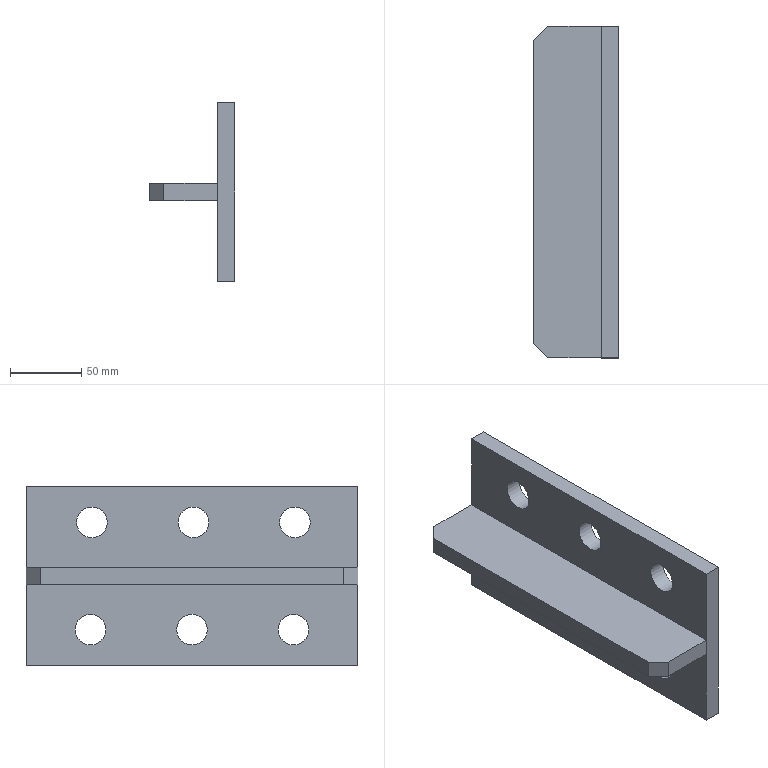Part | STEP file | PN_0039 web-top 12t steel corbel_Default<As Machined> | 2 solids | 20 faces | box 59.5 x 232 x 125 mm | volume 452900 mm3 | plane 14 | cylinder 6 | commonest cylinder face diameters 21.5 x6
STEP:
#1=CARTESIAN_POINT('',(0.,0.,0.));
#2=DIRECTION('',(0.,0.,1.));
#3=DIRECTION('',(1.,0.,0.));
#4=AXIS2_PLACEMENT_3D('',#1,#2,#3);
#5=CARTESIAN_POINT('',(23.75,-115.,-56.496));
#6=VERTEX_POINT('',#5);
#7=CARTESIAN_POINT('',(23.75,117.,-56.496));
#8=VERTEX_POINT('',#7);
#9=CARTESIAN_POINT('',(23.75,117.,-56.496));
#10=DIRECTION('',(0.,1.,0.));
#11=VECTOR('',#10,1.);
#12=LINE('',#9,#11);
#13=CARTESIAN_POINT('',(35.75,117.,-56.496));
#14=DIRECTION('',(0.,0.,1.));
#15=DIRECTION('',(0.,-1.,0.));
#16=AXIS2_PLACEMENT_3D('',#13,#14,#15);
#17=PLANE('',#16);
#18=CARTESIAN_POINT('',(0.,-12.));
#19=DIRECTION('',(-1.,0.));
#20=VECTOR('',#19,1.);
#21=LINE('',#18,#20);
#22=(GEOMETRIC_REPRESENTATION_CONTEXT(2)PARAMETRIC_REPRESENTATION_CONTEXT()REPRESENTATION_CONTEXT('',''));
#23=DEFINITIONAL_REPRESENTATION('',(#21),#22);
#24=PCURVE('',#17,#23);
#25=CARTESIAN_POINT('',(23.75,-17.06,106.06));
#26=DIRECTION('',(1.,0.,0.));
#27=DIRECTION('',(0.,0.,-1.));
#28=AXIS2_PLACEMENT_3D('',#25,#26,#27);
#29=PLANE('',#28);
#30=CARTESIAN_POINT('',(162.556,134.06));
#31=DIRECTION('',(0.,1.));
#32=VECTOR('',#31,1.);
#33=LINE('',#30,#32);
#34=(GEOMETRIC_REPRESENTATION_CONTEXT(2)PARAMETRIC_REPRESENTATION_CONTEXT()REPRESENTATION_CONTEXT('',''));
#35=DEFINITIONAL_REPRESENTATION('',(#33),#34);
#36=PCURVE('',#29,#35);
#37=SURFACE_CURVE('',#12,(#24,#36),.PCURVE_S1.);
#38=EDGE_CURVE('',#6,#8,#37,.T.);
#39=ORIENTED_EDGE('',*,*,#38,.T.);
#40=CARTESIAN_POINT('',(35.75,117.,-56.496));
#41=VERTEX_POINT('',#40);
#42=CARTESIAN_POINT('',(35.75,117.,-56.496));
#43=DIRECTION('',(-1.,0.,0.));
#44=VECTOR('',#43,1.);
#45=LINE('',#42,#44);
#46=CARTESIAN_POINT('',(0.,0.));
#47=DIRECTION('',(0.,-1.));
#48=VECTOR('',#47,1.);
#49=LINE('',#46,#48);
#50=(GEOMETRIC_REPRESENTATION_CONTEXT(2)PARAMETRIC_REPRESENTATION_CONTEXT()REPRESENTATION_CONTEXT('',''));
#51=DEFINITIONAL_REPRESENTATION('',(#49),#50);
#52=PCURVE('',#17,#51);
#53=CARTESIAN_POINT('',(35.75,117.,68.504));
#54=DIRECTION('',(0.,-1.,0.));
#55=DIRECTION('',(0.,0.,-1.));
#56=AXIS2_PLACEMENT_3D('',#53,#54,#55);
#57=PLANE('',#56);
#58=CARTESIAN_POINT('',(125.,0.));
#59=DIRECTION('',(0.,-1.));
#60=VECTOR('',#59,1.);
#61=LINE('',#58,#60);
#62=(GEOMETRIC_REPRESENTATION_CONTEXT(2)PARAMETRIC_REPRESENTATION_CONTEXT()REPRESENTATION_CONTEXT('',''));
#63=DEFINITIONAL_REPRESENTATION('',(#61),#62);
#64=PCURVE('',#57,#63);
#65=SURFACE_CURVE('',#45,(#52,#64),.PCURVE_S1.);
#66=EDGE_CURVE('',#41,#8,#65,.T.);
#67=ORIENTED_EDGE('',*,*,#66,.F.);
#68=CARTESIAN_POINT('',(35.75,-115.,-56.496));
#69=VERTEX_POINT('',#68);
#70=CARTESIAN_POINT('',(35.75,117.,-56.496));
#71=DIRECTION('',(0.,1.,0.));
#72=VECTOR('',#71,1.);
#73=LINE('',#70,#72);
#74=CARTESIAN_POINT('',(0.,0.));
#75=DIRECTION('',(-1.,0.));
#76=VECTOR('',#75,1.);
#77=LINE('',#74,#76);
#78=(GEOMETRIC_REPRESENTATION_CONTEXT(2)PARAMETRIC_REPRESENTATION_CONTEXT()REPRESENTATION_CONTEXT('',''));
#79=DEFINITIONAL_REPRESENTATION('',(#77),#78);
#80=PCURVE('',#17,#79);
#81=CARTESIAN_POINT('',(35.75,-17.06,106.06));
#82=DIRECTION('',(1.,0.,0.));
#83=DIRECTION('',(0.,0.,-1.));
#84=AXIS2_PLACEMENT_3D('',#81,#82,#83);
#85=PLANE('',#84);
#86=CARTESIAN_POINT('',(162.556,134.06));
#87=DIRECTION('',(0.,1.));
#88=VECTOR('',#87,1.);
#89=LINE('',#86,#88);
#90=(GEOMETRIC_REPRESENTATION_CONTEXT(2)PARAMETRIC_REPRESENTATION_CONTEXT()REPRESENTATION_CONTEXT('',''));
#91=DEFINITIONAL_REPRESENTATION('',(#89),#90);
#92=PCURVE('',#85,#91);
#93=SURFACE_CURVE('',#73,(#80,#92),.PCURVE_S1.);
#94=EDGE_CURVE('',#69,#41,#93,.T.);
#95=ORIENTED_EDGE('',*,*,#94,.F.);
#96=CARTESIAN_POINT('',(35.75,-115.,-56.496));
#97=DIRECTION('',(-1.,0.,0.));
#98=VECTOR('',#97,1.);
#99=LINE('',#96,#98);
#100=CARTESIAN_POINT('',(232.,0.));
#101=DIRECTION('',(0.,-1.));
#102=VECTOR('',#101,1.);
#103=LINE('',#100,#102);
#104=(GEOMETRIC_REPRESENTATION_CONTEXT(2)PARAMETRIC_REPRESENTATION_CONTEXT()REPRESENTATION_CONTEXT('',''));
#105=DEFINITIONAL_REPRESENTATION('',(#103),#104);
#106=PCURVE('',#17,#105);
#107=CARTESIAN_POINT('',(35.75,-115.,68.504));
#108=DIRECTION('',(0.,1.,0.));
#109=DIRECTION('',(0.,0.,1.));
#110=AXIS2_PLACEMENT_3D('',#107,#108,#109);
#111=PLANE('',#110);
#112=CARTESIAN_POINT('',(-125.,0.));
#113=DIRECTION('',(0.,-1.));
#114=VECTOR('',#113,1.);
#115=LINE('',#112,#114);
#116=(GEOMETRIC_REPRESENTATION_CONTEXT(2)PARAMETRIC_REPRESENTATION_CONTEXT()REPRESENTATION_CONTEXT('',''));
#117=DEFINITIONAL_REPRESENTATION('',(#115),#116);
#118=PCURVE('',#111,#117);
#119=SURFACE_CURVE('',#99,(#106,#118),.PCURVE_S1.);
#120=EDGE_CURVE('',#69,#6,#119,.T.);
#121=ORIENTED_EDGE('',*,*,#120,.T.);
#122=EDGE_LOOP('',(#39,#67,#95,#121));
#123=FACE_BOUND('',#122,.T.);
#124=ADVANCED_FACE('',(#123),#17,.F.);
#125=CARTESIAN_POINT('',(23.75,117.,68.504));
#126=VERTEX_POINT('',#125);
#127=CARTESIAN_POINT('',(23.75,117.,68.504));
#128=DIRECTION('',(0.,0.,1.));
#129=VECTOR('',#128,1.);
#130=LINE('',#127,#129);
#131=CARTESIAN_POINT('',(0.,-12.));
#132=DIRECTION('',(-1.,0.));
#133=VECTOR('',#132,1.);
#134=LINE('',#131,#133);
#135=(GEOMETRIC_REPRESENTATION_CONTEXT(2)PARAMETRIC_REPRESENTATION_CONTEXT()REPRESENTATION_CONTEXT('',''));
#136=DEFINITIONAL_REPRESENTATION('',(#134),#135);
#137=PCURVE('',#57,#136);
#138=CARTESIAN_POINT('',(37.556,134.06));
#139=DIRECTION('',(-1.,0.));
#140=VECTOR('',#139,1.);
#141=LINE('',#138,#140);
#142=(GEOMETRIC_REPRESENTATION_CONTEXT(2)PARAMETRIC_REPRESENTATION_CONTEXT()REPRESENTATION_CONTEXT('',''));
#143=DEFINITIONAL_REPRESENTATION('',(#141),#142);
#144=PCURVE('',#29,#143);
#145=SURFACE_CURVE('',#130,(#137,#144),.PCURVE_S1.);
#146=EDGE_CURVE('',#8,#126,#145,.T.);
#147=ORIENTED_EDGE('',*,*,#146,.T.);
#148=CARTESIAN_POINT('',(35.75,117.,68.504));
#149=VERTEX_POINT('',#148);
#150=CARTESIAN_POINT('',(35.75,117.,68.504));
#151=DIRECTION('',(-1.,0.,0.));
#152=VECTOR('',#151,1.);
#153=LINE('',#150,#152);
#154=CARTESIAN_POINT('',(0.,0.));
#155=DIRECTION('',(0.,-1.));
#156=VECTOR('',#155,1.);
#157=LINE('',#154,#156);
#158=(GEOMETRIC_REPRESENTATION_CONTEXT(2)PARAMETRIC_REPRESENTATION_CONTEXT()REPRESENTATION_CONTEXT('',''));
#159=DEFINITIONAL_REPRESENTATION('',(#157),#158);
#160=PCURVE('',#57,#159);
#161=CARTESIAN_POINT('',(35.75,117.,68.504));
#162=DIRECTION('',(0.,0.,-1.));
#163=DIRECTION('',(0.,1.,0.));
#164=AXIS2_PLACEMENT_3D('',#161,#162,#163);
#165=PLANE('',#164);
#166=CARTESIAN_POINT('',(0.,0.));
#167=DIRECTION('',(0.,-1.));
#168=VECTOR('',#167,1.);
#169=LINE('',#166,#168);
#170=(GEOMETRIC_REPRESENTATION_CONTEXT(2)PARAMETRIC_REPRESENTATION_CONTEXT()REPRESENTATION_CONTEXT('',''));
#171=DEFINITIONAL_REPRESENTATION('',(#169),#170);
#172=PCURVE('',#165,#171);
#173=SURFACE_CURVE('',#153,(#160,#172),.PCURVE_S1.);
#174=EDGE_CURVE('',#149,#126,#173,.T.);
#175=ORIENTED_EDGE('',*,*,#174,.F.);
#176=CARTESIAN_POINT('',(35.75,117.,68.504));
#177=DIRECTION('',(0.,0.,1.));
#178=VECTOR('',#177,1.);
#179=LINE('',#176,#178);
#180=CARTESIAN_POINT('',(0.,0.));
#181=DIRECTION('',(-1.,0.));
#182=VECTOR('',#181,1.);
#183=LINE('',#180,#182);
#184=(GEOMETRIC_REPRESENTATION_CONTEXT(2)PARAMETRIC_REPRESENTATION_CONTEXT()REPRESENTATION_CONTEXT('',''));
#185=DEFINITIONAL_REPRESENTATION('',(#183),#184);
#186=PCURVE('',#57,#185);
#187=CARTESIAN_POINT('',(37.556,134.06));
#188=DIRECTION('',(-1.,0.));
#189=VECTOR('',#188,1.);
#190=LINE('',#187,#189);
#191=(GEOMETRIC_REPRESENTATION_CONTEXT(2)PARAMETRIC_REPRESENTATION_CONTEXT()REPRESENTATION_CONTEXT('',''));
#192=DEFINITIONAL_REPRESENTATION('',(#190),#191);
#193=PCURVE('',#85,#192);
#194=SURFACE_CURVE('',#179,(#186,#193),.PCURVE_S1.);
#195=EDGE_CURVE('',#41,#149,#194,.T.);
#196=ORIENTED_EDGE('',*,*,#195,.F.);
#197=ORIENTED_EDGE('',*,*,#66,.T.);
#198=EDGE_LOOP('',(#147,#175,#196,#197));
#199=FACE_BOUND('',#198,.T.);
#200=ADVANCED_FACE('',(#199),#57,.F.);
#201=CARTESIAN_POINT('',(23.75,-115.,68.504));
#202=VERTEX_POINT('',#201);
#203=CARTESIAN_POINT('',(23.75,117.,68.504));
#204=DIRECTION('',(0.,-1.,0.));
#205=VECTOR('',#204,1.);
#206=LINE('',#203,#205);
#207=CARTESIAN_POINT('',(0.,-12.));
#208=DIRECTION('',(-1.,0.));
#209=VECTOR('',#208,1.);
#210=LINE('',#207,#209);
#211=(GEOMETRIC_REPRESENTATION_CONTEXT(2)PARAMETRIC_REPRESENTATION_CONTEXT()REPRESENTATION_CONTEXT('',''));
#212=DEFINITIONAL_REPRESENTATION('',(#210),#211);
#213=PCURVE('',#165,#212);
#214=CARTESIAN_POINT('',(37.556,134.06));
#215=DIRECTION('',(0.,-1.));
#216=VECTOR('',#215,1.);
#217=LINE('',#214,#216);
#218=(GEOMETRIC_REPRESENTATION_CONTEXT(2)PARAMETRIC_REPRESENTATION_CONTEXT()REPRESENTATION_CONTEXT('',''));
#219=DEFINITIONAL_REPRESENTATION('',(#217),#218);
#220=PCURVE('',#29,#219);
#221=SURFACE_CURVE('',#206,(#213,#220),.PCURVE_S1.);
#222=EDGE_CURVE('',#126,#202,#221,.T.);
#223=ORIENTED_EDGE('',*,*,#222,.T.);
#224=CARTESIAN_POINT('',(35.75,-115.,68.504));
#225=VERTEX_POINT('',#224);
#226=CARTESIAN_POINT('',(35.75,-115.,68.504));
#227=DIRECTION('',(-1.,0.,0.));
#228=VECTOR('',#227,1.);
#229=LINE('',#226,#228);
#230=CARTESIAN_POINT('',(-232.,0.));
#231=DIRECTION('',(0.,-1.));
#232=VECTOR('',#231,1.);
#233=LINE('',#230,#232);
#234=(GEOMETRIC_REPRESENTATION_CONTEXT(2)PARAMETRIC_REPRESENTATION_CONTEXT()REPRESENTATION_CONTEXT('',''));
#235=DEFINITIONAL_REPRESENTATION('',(#233),#234);
#236=PCURVE('',#165,#235);
#237=CARTESIAN_POINT('',(0.,0.));
#238=DIRECTION('',(0.,-1.));
#239=VECTOR('',#238,1.);
#240=LINE('',#237,#239);
#241=(GEOMETRIC_REPRESENTATION_CONTEXT(2)PARAMETRIC_REPRESENTATION_CONTEXT()REPRESENTATION_CONTEXT('',''));
#242=DEFINITIONAL_REPRESENTATION('',(#240),#241);
#243=PCURVE('',#111,#242);
#244=SURFACE_CURVE('',#229,(#236,#243),.PCURVE_S1.);
#245=EDGE_CURVE('',#225,#202,#244,.T.);
#246=ORIENTED_EDGE('',*,*,#245,.F.);
#247=CARTESIAN_POINT('',(35.75,117.,68.504));
#248=DIRECTION('',(0.,-1.,0.));
#249=VECTOR('',#248,1.);
#250=LINE('',#247,#249);
#251=CARTESIAN_POINT('',(0.,0.));
#252=DIRECTION('',(-1.,0.));
#253=VECTOR('',#252,1.);
#254=LINE('',#251,#253);
#255=(GEOMETRIC_REPRESENTATION_CONTEXT(2)PARAMETRIC_REPRESENTATION_CONTEXT()REPRESENTATION_CONTEXT('',''));
#256=DEFINITIONAL_REPRESENTATION('',(#254),#255);
#257=PCURVE('',#165,#256);
#258=CARTESIAN_POINT('',(37.556,134.06));
#259=DIRECTION('',(0.,-1.));
#260=VECTOR('',#259,1.);
#261=LINE('',#258,#260);
#262=(GEOMETRIC_REPRESENTATION_CONTEXT(2)PARAMETRIC_REPRESENTATION_CONTEXT()REPRESENTATION_CONTEXT('',''));
#263=DEFINITIONAL_REPRESENTATION('',(#261),#262);
#264=PCURVE('',#85,#263);
#265=SURFACE_CURVE('',#250,(#257,#264),.PCURVE_S1.);
#266=EDGE_CURVE('',#149,#225,#265,.T.);
#267=ORIENTED_EDGE('',*,*,#266,.F.);
#268=ORIENTED_EDGE('',*,*,#174,.T.);
#269=EDGE_LOOP('',(#223,#246,#267,#268));
#270=FACE_BOUND('',#269,.T.);
#271=ADVANCED_FACE('',(#270),#165,.F.);
#272=CARTESIAN_POINT('',(23.75,-115.,68.504));
#273=DIRECTION('',(0.,0.,-1.));
#274=VECTOR('',#273,1.);
#275=LINE('',#272,#274);
#276=CARTESIAN_POINT('',(0.,-12.));
#277=DIRECTION('',(-1.,0.));
#278=VECTOR('',#277,1.);
#279=LINE('',#276,#278);
#280=(GEOMETRIC_REPRESENTATION_CONTEXT(2)PARAMETRIC_REPRESENTATION_CONTEXT()REPRESENTATION_CONTEXT('',''));
#281=DEFINITIONAL_REPRESENTATION('',(#279),#280);
#282=PCURVE('',#111,#281);
#283=CARTESIAN_POINT('',(37.556,-97.94));
#284=DIRECTION('',(1.,0.));
#285=VECTOR('',#284,1.);
#286=LINE('',#283,#285);
#287=(GEOMETRIC_REPRESENTATION_CONTEXT(2)PARAMETRIC_REPRESENTATION_CONTEXT()REPRESENTATION_CONTEXT('',''));
#288=DEFINITIONAL_REPRESENTATION('',(#286),#287);
#289=PCURVE('',#29,#288);
#290=SURFACE_CURVE('',#275,(#282,#289),.PCURVE_S1.);
#291=EDGE_CURVE('',#202,#6,#290,.T.);
#292=ORIENTED_EDGE('',*,*,#291,.T.);
#293=ORIENTED_EDGE('',*,*,#120,.F.);
#294=CARTESIAN_POINT('',(35.75,-115.,68.504));
#295=DIRECTION('',(0.,0.,-1.));
#296=VECTOR('',#295,1.);
#297=LINE('',#294,#296);
#298=CARTESIAN_POINT('',(0.,0.));
#299=DIRECTION('',(-1.,0.));
#300=VECTOR('',#299,1.);
#301=LINE('',#298,#300);
#302=(GEOMETRIC_REPRESENTATION_CONTEXT(2)PARAMETRIC_REPRESENTATION_CONTEXT()REPRESENTATION_CONTEXT('',''));
#303=DEFINITIONAL_REPRESENTATION('',(#301),#302);
#304=PCURVE('',#111,#303);
#305=CARTESIAN_POINT('',(37.556,-97.94));
#306=DIRECTION('',(1.,0.));
#307=VECTOR('',#306,1.);
#308=LINE('',#305,#307);
#309=(GEOMETRIC_REPRESENTATION_CONTEXT(2)PARAMETRIC_REPRESENTATION_CONTEXT()REPRESENTATION_CONTEXT('',''));
#310=DEFINITIONAL_REPRESENTATION('',(#308),#309);
#311=PCURVE('',#85,#310);
#312=SURFACE_CURVE('',#297,(#304,#311),.PCURVE_S1.);
#313=EDGE_CURVE('',#225,#69,#312,.T.);
#314=ORIENTED_EDGE('',*,*,#313,.F.);
#315=ORIENTED_EDGE('',*,*,#245,.T.);
#316=EDGE_LOOP('',(#292,#293,#314,#315));
#317=FACE_BOUND('',#316,.T.);
#318=ADVANCED_FACE('',(#317),#111,.F.);
#319=CARTESIAN_POINT('',(35.75,71.,32.754));
#320=VERTEX_POINT('',#319);
#321=CARTESIAN_POINT('',(35.75,71.,43.504));
#322=DIRECTION('',(1.,0.,0.));
#323=DIRECTION('',(0.,0.,-1.));
#324=AXIS2_PLACEMENT_3D('',#321,#322,#323);
#325=CIRCLE('',#324,10.75);
#326=CARTESIAN_POINT('',(62.556,88.06));
#327=DIRECTION('',(1.,0.));
#328=AXIS2_PLACEMENT_2D('',#326,#327);
#329=CIRCLE('',#328,10.75);
#330=(GEOMETRIC_REPRESENTATION_CONTEXT(2)PARAMETRIC_REPRESENTATION_CONTEXT()REPRESENTATION_CONTEXT('',''));
#331=DEFINITIONAL_REPRESENTATION('',(#329),#330);
#332=PCURVE('',#85,#331);
#333=CARTESIAN_POINT('',(35.75,71.,43.504));
#334=DIRECTION('',(1.,0.,0.));
#335=DIRECTION('',(0.,0.,-1.));
#336=AXIS2_PLACEMENT_3D('',#333,#334,#335);
#337=CYLINDRICAL_SURFACE('',#336,10.75);
#338=CARTESIAN_POINT('',(0.,0.));
#339=DIRECTION('',(1.,0.));
#340=VECTOR('',#339,1.);
#341=LINE('',#338,#340);
#342=(GEOMETRIC_REPRESENTATION_CONTEXT(2)PARAMETRIC_REPRESENTATION_CONTEXT()REPRESENTATION_CONTEXT('',''));
#343=DEFINITIONAL_REPRESENTATION('',(#341),#342);
#344=PCURVE('',#337,#343);
#345=SURFACE_CURVE('',#325,(#332,#344),.PCURVE_S1.);
#346=EDGE_CURVE('',#320,#320,#345,.T.);
#347=ORIENTED_EDGE('',*,*,#346,.F.);
#348=EDGE_LOOP('',(#347));
#349=FACE_BOUND('',#348,.T.);
#350=CARTESIAN_POINT('',(35.75,0.0001482,32.754));
#351=VERTEX_POINT('',#350);
#352=CARTESIAN_POINT('',(35.75,0.0001482,43.504));
#353=DIRECTION('',(1.,0.,0.));
#354=DIRECTION('',(0.,0.,-1.));
#355=AXIS2_PLACEMENT_3D('',#352,#353,#354);
#356=CIRCLE('',#355,10.75);
#357=CARTESIAN_POINT('',(62.556,17.06));
#358=DIRECTION('',(1.,0.));
#359=AXIS2_PLACEMENT_2D('',#357,#358);
#360=CIRCLE('',#359,10.75);
#361=(GEOMETRIC_REPRESENTATION_CONTEXT(2)PARAMETRIC_REPRESENTATION_CONTEXT()REPRESENTATION_CONTEXT('',''));
#362=DEFINITIONAL_REPRESENTATION('',(#360),#361);
#363=PCURVE('',#85,#362);
#364=CARTESIAN_POINT('',(35.75,0.0001482,43.504));
#365=DIRECTION('',(1.,0.,0.));
#366=DIRECTION('',(0.,0.,-1.));
#367=AXIS2_PLACEMENT_3D('',#364,#365,#366);
#368=CYLINDRICAL_SURFACE('',#367,10.75);
#369=CARTESIAN_POINT('',(0.,0.));
#370=DIRECTION('',(1.,0.));
#371=VECTOR('',#370,1.);
#372=LINE('',#369,#371);
#373=(GEOMETRIC_REPRESENTATION_CONTEXT(2)PARAMETRIC_REPRESENTATION_CONTEXT()REPRESENTATION_CONTEXT('',''));
#374=DEFINITIONAL_REPRESENTATION('',(#372),#373);
#375=PCURVE('',#368,#374);
#376=SURFACE_CURVE('',#356,(#363,#375),.PCURVE_S1.);
#377=EDGE_CURVE('',#351,#351,#376,.T.);
#378=ORIENTED_EDGE('',*,*,#377,.F.);
#379=EDGE_LOOP('',(#378));
#380=FACE_BOUND('',#379,.T.);
#381=CARTESIAN_POINT('',(35.75,1.,-42.246));
#382=VERTEX_POINT('',#381);
#383=CARTESIAN_POINT('',(35.75,1.,-31.496));
#384=DIRECTION('',(1.,0.,0.));
#385=DIRECTION('',(0.,0.,-1.));
#386=AXIS2_PLACEMENT_3D('',#383,#384,#385);
#387=CIRCLE('',#386,10.75);
#388=CARTESIAN_POINT('',(137.556,18.06));
#389=DIRECTION('',(1.,0.));
#390=AXIS2_PLACEMENT_2D('',#388,#389);
#391=CIRCLE('',#390,10.75);
#392=(GEOMETRIC_REPRESENTATION_CONTEXT(2)PARAMETRIC_REPRESENTATION_CONTEXT()REPRESENTATION_CONTEXT('',''));
#393=DEFINITIONAL_REPRESENTATION('',(#391),#392);
#394=PCURVE('',#85,#393);
#395=CARTESIAN_POINT('',(35.75,1.,-31.496));
#396=DIRECTION('',(1.,0.,0.));
#397=DIRECTION('',(0.,0.,-1.));
#398=AXIS2_PLACEMENT_3D('',#395,#396,#397);
#399=CYLINDRICAL_SURFACE('',#398,10.75);
#400=CARTESIAN_POINT('',(0.,0.));
#401=DIRECTION('',(1.,0.));
#402=VECTOR('',#401,1.);
#403=LINE('',#400,#402);
#404=(GEOMETRIC_REPRESENTATION_CONTEXT(2)PARAMETRIC_REPRESENTATION_CONTEXT()REPRESENTATION_CONTEXT('',''));
#405=DEFINITIONAL_REPRESENTATION('',(#403),#404);
#406=PCURVE('',#399,#405);
#407=SURFACE_CURVE('',#387,(#394,#406),.PCURVE_S1.);
#408=EDGE_CURVE('',#382,#382,#407,.T.);
#409=ORIENTED_EDGE('',*,*,#408,.F.);
#410=EDGE_LOOP('',(#409));
#411=FACE_BOUND('',#410,.T.);
#412=CARTESIAN_POINT('',(35.75,72.,-42.246));
#413=VERTEX_POINT('',#412);
#414=CARTESIAN_POINT('',(35.75,72.,-31.496));
#415=DIRECTION('',(1.,0.,0.));
#416=DIRECTION('',(0.,0.,-1.));
#417=AXIS2_PLACEMENT_3D('',#414,#415,#416);
#418=CIRCLE('',#417,10.75);
#419=CARTESIAN_POINT('',(137.556,89.06));
#420=DIRECTION('',(1.,0.));
#421=AXIS2_PLACEMENT_2D('',#419,#420);
#422=CIRCLE('',#421,10.75);
#423=(GEOMETRIC_REPRESENTATION_CONTEXT(2)PARAMETRIC_REPRESENTATION_CONTEXT()REPRESENTATION_CONTEXT('',''));
#424=DEFINITIONAL_REPRESENTATION('',(#422),#423);
#425=PCURVE('',#85,#424);
#426=CARTESIAN_POINT('',(35.75,72.,-31.496));
#427=DIRECTION('',(1.,0.,0.));
#428=DIRECTION('',(0.,0.,-1.));
#429=AXIS2_PLACEMENT_3D('',#426,#427,#428);
#430=CYLINDRICAL_SURFACE('',#429,10.75);
#431=CARTESIAN_POINT('',(0.,0.));
#432=DIRECTION('',(1.,0.));
#433=VECTOR('',#432,1.);
#434=LINE('',#431,#433);
#435=(GEOMETRIC_REPRESENTATION_CONTEXT(2)PARAMETRIC_REPRESENTATION_CONTEXT()REPRESENTATION_CONTEXT('',''));
#436=DEFINITIONAL_REPRESENTATION('',(#434),#435);
#437=PCURVE('',#430,#436);
#438=SURFACE_CURVE('',#418,(#425,#437),.PCURVE_S1.);
#439=EDGE_CURVE('',#413,#413,#438,.T.);
#440=ORIENTED_EDGE('',*,*,#439,.F.);
#441=EDGE_LOOP('',(#440));
#442=FACE_BOUND('',#441,.T.);
#443=CARTESIAN_POINT('',(35.75,-71.,32.754));
#444=VERTEX_POINT('',#443);
#445=CARTESIAN_POINT('',(35.75,-71.,43.504));
#446=DIRECTION('',(1.,0.,0.));
#447=DIRECTION('',(0.,0.,-1.));
#448=AXIS2_PLACEMENT_3D('',#445,#446,#447);
#449=CIRCLE('',#448,10.75);
#450=CARTESIAN_POINT('',(62.556,-53.94));
#451=DIRECTION('',(1.,0.));
#452=AXIS2_PLACEMENT_2D('',#450,#451);
#453=CIRCLE('',#452,10.75);
#454=(GEOMETRIC_REPRESENTATION_CONTEXT(2)PARAMETRIC_REPRESENTATION_CONTEXT()REPRESENTATION_CONTEXT('',''));
#455=DEFINITIONAL_REPRESENTATION('',(#453),#454);
#456=PCURVE('',#85,#455);
#457=CARTESIAN_POINT('',(35.75,-71.,43.504));
#458=DIRECTION('',(1.,0.,0.));
#459=DIRECTION('',(0.,0.,-1.));
#460=AXIS2_PLACEMENT_3D('',#457,#458,#459);
#461=CYLINDRICAL_SURFACE('',#460,10.75);
#462=CARTESIAN_POINT('',(0.,0.));
#463=DIRECTION('',(1.,0.));
#464=VECTOR('',#463,1.);
#465=LINE('',#462,#464);
#466=(GEOMETRIC_REPRESENTATION_CONTEXT(2)PARAMETRIC_REPRESENTATION_CONTEXT()REPRESENTATION_CONTEXT('',''));
#467=DEFINITIONAL_REPRESENTATION('',(#465),#466);
#468=PCURVE('',#461,#467);
#469=SURFACE_CURVE('',#449,(#456,#468),.PCURVE_S1.);
#470=EDGE_CURVE('',#444,#444,#469,.T.);
#471=ORIENTED_EDGE('',*,*,#470,.F.);
#472=EDGE_LOOP('',(#471));
#473=FACE_BOUND('',#472,.T.);
#474=CARTESIAN_POINT('',(35.75,-70.,-42.246));
#475=VERTEX_POINT('',#474);
#476=CARTESIAN_POINT('',(35.75,-70.,-31.496));
#477=DIRECTION('',(1.,0.,0.));
#478=DIRECTION('',(0.,0.,-1.));
#479=AXIS2_PLACEMENT_3D('',#476,#477,#478);
#480=CIRCLE('',#479,10.75);
#481=CARTESIAN_POINT('',(137.556,-52.94));
#482=DIRECTION('',(1.,0.));
#483=AXIS2_PLACEMENT_2D('',#481,#482);
#484=CIRCLE('',#483,10.75);
#485=(GEOMETRIC_REPRESENTATION_CONTEXT(2)PARAMETRIC_REPRESENTATION_CONTEXT()REPRESENTATION_CONTEXT('',''));
#486=DEFINITIONAL_REPRESENTATION('',(#484),#485);
#487=PCURVE('',#85,#486);
#488=CARTESIAN_POINT('',(35.75,-70.,-31.496));
#489=DIRECTION('',(1.,0.,0.));
#490=DIRECTION('',(0.,0.,-1.));
#491=AXIS2_PLACEMENT_3D('',#488,#489,#490);
#492=CYLINDRICAL_SURFACE('',#491,10.75);
#493=CARTESIAN_POINT('',(0.,0.));
#494=DIRECTION('',(1.,0.));
#495=VECTOR('',#494,1.);
#496=LINE('',#493,#495);
#497=(GEOMETRIC_REPRESENTATION_CONTEXT(2)PARAMETRIC_REPRESENTATION_CONTEXT()REPRESENTATION_CONTEXT('',''));
#498=DEFINITIONAL_REPRESENTATION('',(#496),#497);
#499=PCURVE('',#492,#498);
#500=SURFACE_CURVE('',#480,(#487,#499),.PCURVE_S1.);
#501=EDGE_CURVE('',#475,#475,#500,.T.);
#502=ORIENTED_EDGE('',*,*,#501,.F.);
#503=EDGE_LOOP('',(#502));
#504=FACE_BOUND('',#503,.T.);
#505=ORIENTED_EDGE('',*,*,#94,.T.);
#506=ORIENTED_EDGE('',*,*,#195,.T.);
#507=ORIENTED_EDGE('',*,*,#266,.T.);
#508=ORIENTED_EDGE('',*,*,#313,.T.);
#509=EDGE_LOOP('',(#505,#506,#507,#508));
#510=FACE_BOUND('',#509,.T.);
#511=ADVANCED_FACE('',(#349,#380,#411,#442,#473,#504,#510),#85,.T.);
#512=CARTESIAN_POINT('',(23.75,71.,32.754));
#513=VERTEX_POINT('',#512);
#514=CARTESIAN_POINT('',(23.75,71.,43.504));
#515=DIRECTION('',(1.,0.,0.));
#516=DIRECTION('',(0.,0.,-1.));
#517=AXIS2_PLACEMENT_3D('',#514,#515,#516);
#518=CIRCLE('',#517,10.75);
#519=CARTESIAN_POINT('',(62.556,88.06));
#520=DIRECTION('',(1.,0.));
#521=AXIS2_PLACEMENT_2D('',#519,#520);
#522=CIRCLE('',#521,10.75);
#523=(GEOMETRIC_REPRESENTATION_CONTEXT(2)PARAMETRIC_REPRESENTATION_CONTEXT()REPRESENTATION_CONTEXT('',''));
#524=DEFINITIONAL_REPRESENTATION('',(#522),#523);
#525=PCURVE('',#29,#524);
#526=CARTESIAN_POINT('',(0.,-12.));
#527=DIRECTION('',(1.,0.));
#528=VECTOR('',#527,1.);
#529=LINE('',#526,#528);
#530=(GEOMETRIC_REPRESENTATION_CONTEXT(2)PARAMETRIC_REPRESENTATION_CONTEXT()REPRESENTATION_CONTEXT('',''));
#531=DEFINITIONAL_REPRESENTATION('',(#529),#530);
#532=PCURVE('',#337,#531);
#533=SURFACE_CURVE('',#518,(#525,#532),.PCURVE_S1.);
#534=EDGE_CURVE('',#513,#513,#533,.T.);
#535=ORIENTED_EDGE('',*,*,#534,.T.);
#536=EDGE_LOOP('',(#535));
#537=FACE_BOUND('',#536,.T.);
#538=CARTESIAN_POINT('',(23.75,0.0001482,32.754));
#539=VERTEX_POINT('',#538);
#540=CARTESIAN_POINT('',(23.75,0.0001482,43.504));
#541=DIRECTION('',(1.,0.,0.));
#542=DIRECTION('',(0.,0.,-1.));
#543=AXIS2_PLACEMENT_3D('',#540,#541,#542);
#544=CIRCLE('',#543,10.75);
#545=CARTESIAN_POINT('',(62.556,17.06));
#546=DIRECTION('',(1.,0.));
#547=AXIS2_PLACEMENT_2D('',#545,#546);
#548=CIRCLE('',#547,10.75);
#549=(GEOMETRIC_REPRESENTATION_CONTEXT(2)PARAMETRIC_REPRESENTATION_CONTEXT()REPRESENTATION_CONTEXT('',''));
#550=DEFINITIONAL_REPRESENTATION('',(#548),#549);
#551=PCURVE('',#29,#550);
#552=CARTESIAN_POINT('',(0.,-12.));
#553=DIRECTION('',(1.,0.));
#554=VECTOR('',#553,1.);
#555=LINE('',#552,#554);
#556=(GEOMETRIC_REPRESENTATION_CONTEXT(2)PARAMETRIC_REPRESENTATION_CONTEXT()REPRESENTATION_CONTEXT('',''));
#557=DEFINITIONAL_REPRESENTATION('',(#555),#556);
#558=PCURVE('',#368,#557);
#559=SURFACE_CURVE('',#544,(#551,#558),.PCURVE_S1.);
#560=EDGE_CURVE('',#539,#539,#559,.T.);
#561=ORIENTED_EDGE('',*,*,#560,.T.);
#562=EDGE_LOOP('',(#561));
#563=FACE_BOUND('',#562,.T.);
#564=CARTESIAN_POINT('',(23.75,1.,-42.246));
#565=VERTEX_POINT('',#564);
#566=CARTESIAN_POINT('',(23.75,1.,-31.496));
#567=DIRECTION('',(1.,0.,0.));
#568=DIRECTION('',(0.,0.,-1.));
#569=AXIS2_PLACEMENT_3D('',#566,#567,#568);
#570=CIRCLE('',#569,10.75);
#571=CARTESIAN_POINT('',(137.556,18.06));
#572=DIRECTION('',(1.,0.));
#573=AXIS2_PLACEMENT_2D('',#571,#572);
#574=CIRCLE('',#573,10.75);
#575=(GEOMETRIC_REPRESENTATION_CONTEXT(2)PARAMETRIC_REPRESENTATION_CONTEXT()REPRESENTATION_CONTEXT('',''));
#576=DEFINITIONAL_REPRESENTATION('',(#574),#575);
#577=PCURVE('',#29,#576);
#578=CARTESIAN_POINT('',(0.,-12.));
#579=DIRECTION('',(1.,0.));
#580=VECTOR('',#579,1.);
#581=LINE('',#578,#580);
#582=(GEOMETRIC_REPRESENTATION_CONTEXT(2)PARAMETRIC_REPRESENTATION_CONTEXT()REPRESENTATION_CONTEXT('',''));
#583=DEFINITIONAL_REPRESENTATION('',(#581),#582);
#584=PCURVE('',#399,#583);
#585=SURFACE_CURVE('',#570,(#577,#584),.PCURVE_S1.);
#586=EDGE_CURVE('',#565,#565,#585,.T.);
#587=ORIENTED_EDGE('',*,*,#586,.T.);
#588=EDGE_LOOP('',(#587));
#589=FACE_BOUND('',#588,.T.);
#590=CARTESIAN_POINT('',(23.75,72.,-42.246));
#591=VERTEX_POINT('',#590);
#592=CARTESIAN_POINT('',(23.75,72.,-31.496));
#593=DIRECTION('',(1.,0.,0.));
#594=DIRECTION('',(0.,0.,-1.));
#595=AXIS2_PLACEMENT_3D('',#592,#593,#594);
#596=CIRCLE('',#595,10.75);
#597=CARTESIAN_POINT('',(137.556,89.06));
#598=DIRECTION('',(1.,0.));
#599=AXIS2_PLACEMENT_2D('',#597,#598);
#600=CIRCLE('',#599,10.75);
#601=(GEOMETRIC_REPRESENTATION_CONTEXT(2)PARAMETRIC_REPRESENTATION_CONTEXT()REPRESENTATION_CONTEXT('',''));
#602=DEFINITIONAL_REPRESENTATION('',(#600),#601);
#603=PCURVE('',#29,#602);
#604=CARTESIAN_POINT('',(0.,-12.));
#605=DIRECTION('',(1.,0.));
#606=VECTOR('',#605,1.);
#607=LINE('',#604,#606);
#608=(GEOMETRIC_REPRESENTATION_CONTEXT(2)PARAMETRIC_REPRESENTATION_CONTEXT()REPRESENTATION_CONTEXT('',''));
#609=DEFINITIONAL_REPRESENTATION('',(#607),#608);
#610=PCURVE('',#430,#609);
#611=SURFACE_CURVE('',#596,(#603,#610),.PCURVE_S1.);
#612=EDGE_CURVE('',#591,#591,#611,.T.);
#613=ORIENTED_EDGE('',*,*,#612,.T.);
#614=EDGE_LOOP('',(#613));
#615=FACE_BOUND('',#614,.T.);
#616=CARTESIAN_POINT('',(23.75,-71.,32.754));
#617=VERTEX_POINT('',#616);
#618=CARTESIAN_POINT('',(23.75,-71.,43.504));
#619=DIRECTION('',(1.,0.,0.));
#620=DIRECTION('',(0.,0.,-1.));
#621=AXIS2_PLACEMENT_3D('',#618,#619,#620);
#622=CIRCLE('',#621,10.75);
#623=CARTESIAN_POINT('',(62.556,-53.94));
#624=DIRECTION('',(1.,0.));
#625=AXIS2_PLACEMENT_2D('',#623,#624);
#626=CIRCLE('',#625,10.75);
#627=(GEOMETRIC_REPRESENTATION_CONTEXT(2)PARAMETRIC_REPRESENTATION_CONTEXT()REPRESENTATION_CONTEXT('',''));
#628=DEFINITIONAL_REPRESENTATION('',(#626),#627);
#629=PCURVE('',#29,#628);
#630=CARTESIAN_POINT('',(0.,-12.));
#631=DIRECTION('',(1.,0.));
#632=VECTOR('',#631,1.);
#633=LINE('',#630,#632);
#634=(GEOMETRIC_REPRESENTATION_CONTEXT(2)PARAMETRIC_REPRESENTATION_CONTEXT()REPRESENTATION_CONTEXT('',''));
#635=DEFINITIONAL_REPRESENTATION('',(#633),#634);
#636=PCURVE('',#461,#635);
#637=SURFACE_CURVE('',#622,(#629,#636),.PCURVE_S1.);
#638=EDGE_CURVE('',#617,#617,#637,.T.);
#639=ORIENTED_EDGE('',*,*,#638,.T.);
#640=EDGE_LOOP('',(#639));
#641=FACE_BOUND('',#640,.T.);
#642=CARTESIAN_POINT('',(23.75,-70.,-42.246));
#643=VERTEX_POINT('',#642);
#644=CARTESIAN_POINT('',(23.75,-70.,-31.496));
#645=DIRECTION('',(1.,0.,0.));
#646=DIRECTION('',(0.,0.,-1.));
#647=AXIS2_PLACEMENT_3D('',#644,#645,#646);
#648=CIRCLE('',#647,10.75);
#649=CARTESIAN_POINT('',(137.556,-52.94));
#650=DIRECTION('',(1.,0.));
#651=AXIS2_PLACEMENT_2D('',#649,#650);
#652=CIRCLE('',#651,10.75);
#653=(GEOMETRIC_REPRESENTATION_CONTEXT(2)PARAMETRIC_REPRESENTATION_CONTEXT()REPRESENTATION_CONTEXT('',''));
#654=DEFINITIONAL_REPRESENTATION('',(#652),#653);
#655=PCURVE('',#29,#654);
#656=CARTESIAN_POINT('',(0.,-12.));
#657=DIRECTION('',(1.,0.));
#658=VECTOR('',#657,1.);
#659=LINE('',#656,#658);
#660=(GEOMETRIC_REPRESENTATION_CONTEXT(2)PARAMETRIC_REPRESENTATION_CONTEXT()REPRESENTATION_CONTEXT('',''));
#661=DEFINITIONAL_REPRESENTATION('',(#659),#660);
#662=PCURVE('',#492,#661);
#663=SURFACE_CURVE('',#648,(#655,#662),.PCURVE_S1.);
#664=EDGE_CURVE('',#643,#643,#663,.T.);
#665=ORIENTED_EDGE('',*,*,#664,.T.);
#666=EDGE_LOOP('',(#665));
#667=FACE_BOUND('',#666,.T.);
#668=ORIENTED_EDGE('',*,*,#38,.F.);
#669=ORIENTED_EDGE('',*,*,#291,.F.);
#670=ORIENTED_EDGE('',*,*,#222,.F.);
#671=ORIENTED_EDGE('',*,*,#146,.F.);
#672=EDGE_LOOP('',(#668,#669,#670,#671));
#673=FACE_BOUND('',#672,.T.);
#674=ADVANCED_FACE('',(#537,#563,#589,#615,#641,#667,#673),#29,.F.);
#675=ORIENTED_EDGE('',*,*,#501,.F.);
#676=CARTESIAN_POINT('',(23.75,-70.,-42.246));
#677=CARTESIAN_POINT('',(35.75,-70.,-42.246));
#678=B_SPLINE_CURVE_WITH_KNOTS('',1,(#676,#677),.UNSPECIFIED.,.F.,.F.,(2,2),(-12.,0.),.PIECEWISE_BEZIER_KNOTS.);
#679=CARTESIAN_POINT('',(0.,0.));
#680=DIRECTION('',(0.,1.));
#681=VECTOR('',#680,1.);
#682=LINE('',#679,#681);
#683=(GEOMETRIC_REPRESENTATION_CONTEXT(2)PARAMETRIC_REPRESENTATION_CONTEXT()REPRESENTATION_CONTEXT('',''));
#684=DEFINITIONAL_REPRESENTATION('',(#682),#683);
#685=PCURVE('',#492,#684);
#686=CARTESIAN_POINT('',(6.283,0.));
#687=DIRECTION('',(0.,1.));
#688=VECTOR('',#687,1.);
#689=LINE('',#686,#688);
#690=(GEOMETRIC_REPRESENTATION_CONTEXT(2)PARAMETRIC_REPRESENTATION_CONTEXT()REPRESENTATION_CONTEXT('',''));
#691=DEFINITIONAL_REPRESENTATION('',(#689),#690);
#692=PCURVE('',#492,#691);
#693=SEAM_CURVE('',#678,(#685,#692),.PCURVE_S1.);
#694=EDGE_CURVE('',#643,#475,#693,.T.);
#695=ORIENTED_EDGE('',*,*,#694,.F.);
#696=ORIENTED_EDGE('',*,*,#664,.T.);
#697=ORIENTED_EDGE('',*,*,#694,.T.);
#698=EDGE_LOOP('',(#675,#695,#696,#697));
#699=FACE_BOUND('',#698,.F.);
#700=ADVANCED_FACE('',(#699),#492,.F.);
#701=ORIENTED_EDGE('',*,*,#470,.F.);
#702=CARTESIAN_POINT('',(23.75,-71.,32.754));
#703=CARTESIAN_POINT('',(35.75,-71.,32.754));
#704=B_SPLINE_CURVE_WITH_KNOTS('',1,(#702,#703),.UNSPECIFIED.,.F.,.F.,(2,2),(-12.,0.),.PIECEWISE_BEZIER_KNOTS.);
#705=CARTESIAN_POINT('',(0.,0.));
#706=DIRECTION('',(0.,1.));
#707=VECTOR('',#706,1.);
#708=LINE('',#705,#707);
#709=(GEOMETRIC_REPRESENTATION_CONTEXT(2)PARAMETRIC_REPRESENTATION_CONTEXT()REPRESENTATION_CONTEXT('',''));
#710=DEFINITIONAL_REPRESENTATION('',(#708),#709);
#711=PCURVE('',#461,#710);
#712=CARTESIAN_POINT('',(6.283,0.));
#713=DIRECTION('',(0.,1.));
#714=VECTOR('',#713,1.);
#715=LINE('',#712,#714);
#716=(GEOMETRIC_REPRESENTATION_CONTEXT(2)PARAMETRIC_REPRESENTATION_CONTEXT()REPRESENTATION_CONTEXT('',''));
#717=DEFINITIONAL_REPRESENTATION('',(#715),#716);
#718=PCURVE('',#461,#717);
#719=SEAM_CURVE('',#704,(#711,#718),.PCURVE_S1.);
#720=EDGE_CURVE('',#617,#444,#719,.T.);
#721=ORIENTED_EDGE('',*,*,#720,.F.);
#722=ORIENTED_EDGE('',*,*,#638,.T.);
#723=ORIENTED_EDGE('',*,*,#720,.T.);
#724=EDGE_LOOP('',(#701,#721,#722,#723));
#725=FACE_BOUND('',#724,.F.);
#726=ADVANCED_FACE('',(#725),#461,.F.);
#727=ORIENTED_EDGE('',*,*,#439,.F.);
#728=CARTESIAN_POINT('',(23.75,72.,-42.246));
#729=CARTESIAN_POINT('',(35.75,72.,-42.246));
#730=B_SPLINE_CURVE_WITH_KNOTS('',1,(#728,#729),.UNSPECIFIED.,.F.,.F.,(2,2),(-12.,0.),.PIECEWISE_BEZIER_KNOTS.);
#731=CARTESIAN_POINT('',(0.,0.));
#732=DIRECTION('',(0.,1.));
#733=VECTOR('',#732,1.);
#734=LINE('',#731,#733);
#735=(GEOMETRIC_REPRESENTATION_CONTEXT(2)PARAMETRIC_REPRESENTATION_CONTEXT()REPRESENTATION_CONTEXT('',''));
#736=DEFINITIONAL_REPRESENTATION('',(#734),#735);
#737=PCURVE('',#430,#736);
#738=CARTESIAN_POINT('',(6.283,0.));
#739=DIRECTION('',(0.,1.));
#740=VECTOR('',#739,1.);
#741=LINE('',#738,#740);
#742=(GEOMETRIC_REPRESENTATION_CONTEXT(2)PARAMETRIC_REPRESENTATION_CONTEXT()REPRESENTATION_CONTEXT('',''));
#743=DEFINITIONAL_REPRESENTATION('',(#741),#742);
#744=PCURVE('',#430,#743);
#745=SEAM_CURVE('',#730,(#737,#744),.PCURVE_S1.);
#746=EDGE_CURVE('',#591,#413,#745,.T.);
#747=ORIENTED_EDGE('',*,*,#746,.F.);
#748=ORIENTED_EDGE('',*,*,#612,.T.);
#749=ORIENTED_EDGE('',*,*,#746,.T.);
#750=EDGE_LOOP('',(#727,#747,#748,#749));
#751=FACE_BOUND('',#750,.F.);
#752=ADVANCED_FACE('',(#751),#430,.F.);
#753=ORIENTED_EDGE('',*,*,#408,.F.);
#754=CARTESIAN_POINT('',(23.75,1.,-42.246));
#755=CARTESIAN_POINT('',(35.75,1.,-42.246));
#756=B_SPLINE_CURVE_WITH_KNOTS('',1,(#754,#755),.UNSPECIFIED.,.F.,.F.,(2,2),(-12.,0.),.PIECEWISE_BEZIER_KNOTS.);
#757=CARTESIAN_POINT('',(0.,0.));
#758=DIRECTION('',(0.,1.));
#759=VECTOR('',#758,1.);
#760=LINE('',#757,#759);
#761=(GEOMETRIC_REPRESENTATION_CONTEXT(2)PARAMETRIC_REPRESENTATION_CONTEXT()REPRESENTATION_CONTEXT('',''));
#762=DEFINITIONAL_REPRESENTATION('',(#760),#761);
#763=PCURVE('',#399,#762);
#764=CARTESIAN_POINT('',(6.283,0.));
#765=DIRECTION('',(0.,1.));
#766=VECTOR('',#765,1.);
#767=LINE('',#764,#766);
#768=(GEOMETRIC_REPRESENTATION_CONTEXT(2)PARAMETRIC_REPRESENTATION_CONTEXT()REPRESENTATION_CONTEXT('',''));
#769=DEFINITIONAL_REPRESENTATION('',(#767),#768);
#770=PCURVE('',#399,#769);
#771=SEAM_CURVE('',#756,(#763,#770),.PCURVE_S1.);
#772=EDGE_CURVE('',#565,#382,#771,.T.);
#773=ORIENTED_EDGE('',*,*,#772,.F.);
#774=ORIENTED_EDGE('',*,*,#586,.T.);
#775=ORIENTED_EDGE('',*,*,#772,.T.);
#776=EDGE_LOOP('',(#753,#773,#774,#775));
#777=FACE_BOUND('',#776,.F.);
#778=ADVANCED_FACE('',(#777),#399,.F.);
#779=ORIENTED_EDGE('',*,*,#377,.F.);
#780=CARTESIAN_POINT('',(23.75,0.0001482,32.754));
#781=CARTESIAN_POINT('',(35.75,0.0001482,32.754));
#782=B_SPLINE_CURVE_WITH_KNOTS('',1,(#780,#781),.UNSPECIFIED.,.F.,.F.,(2,2),(-12.,0.),.PIECEWISE_BEZIER_KNOTS.);
#783=CARTESIAN_POINT('',(0.,0.));
#784=DIRECTION('',(0.,1.));
#785=VECTOR('',#784,1.);
#786=LINE('',#783,#785);
#787=(GEOMETRIC_REPRESENTATION_CONTEXT(2)PARAMETRIC_REPRESENTATION_CONTEXT()REPRESENTATION_CONTEXT('',''));
#788=DEFINITIONAL_REPRESENTATION('',(#786),#787);
#789=PCURVE('',#368,#788);
#790=CARTESIAN_POINT('',(6.283,0.));
#791=DIRECTION('',(0.,1.));
#792=VECTOR('',#791,1.);
#793=LINE('',#790,#792);
#794=(GEOMETRIC_REPRESENTATION_CONTEXT(2)PARAMETRIC_REPRESENTATION_CONTEXT()REPRESENTATION_CONTEXT('',''));
#795=DEFINITIONAL_REPRESENTATION('',(#793),#794);
#796=PCURVE('',#368,#795);
#797=SEAM_CURVE('',#782,(#789,#796),.PCURVE_S1.);
#798=EDGE_CURVE('',#539,#351,#797,.T.);
#799=ORIENTED_EDGE('',*,*,#798,.F.);
#800=ORIENTED_EDGE('',*,*,#560,.T.);
#801=ORIENTED_EDGE('',*,*,#798,.T.);
#802=EDGE_LOOP('',(#779,#799,#800,#801));
#803=FACE_BOUND('',#802,.F.);
#804=ADVANCED_FACE('',(#803),#368,.F.);
#805=ORIENTED_EDGE('',*,*,#346,.F.);
#806=CARTESIAN_POINT('',(23.75,71.,32.754));
#807=CARTESIAN_POINT('',(35.75,71.,32.754));
#808=B_SPLINE_CURVE_WITH_KNOTS('',1,(#806,#807),.UNSPECIFIED.,.F.,.F.,(2,2),(-12.,0.),.PIECEWISE_BEZIER_KNOTS.);
#809=CARTESIAN_POINT('',(0.,0.));
#810=DIRECTION('',(0.,1.));
#811=VECTOR('',#810,1.);
#812=LINE('',#809,#811);
#813=(GEOMETRIC_REPRESENTATION_CONTEXT(2)PARAMETRIC_REPRESENTATION_CONTEXT()REPRESENTATION_CONTEXT('',''));
#814=DEFINITIONAL_REPRESENTATION('',(#812),#813);
#815=PCURVE('',#337,#814);
#816=CARTESIAN_POINT('',(6.283,0.));
#817=DIRECTION('',(0.,1.));
#818=VECTOR('',#817,1.);
#819=LINE('',#816,#818);
#820=(GEOMETRIC_REPRESENTATION_CONTEXT(2)PARAMETRIC_REPRESENTATION_CONTEXT()REPRESENTATION_CONTEXT('',''));
#821=DEFINITIONAL_REPRESENTATION('',(#819),#820);
#822=PCURVE('',#337,#821);
#823=SEAM_CURVE('',#808,(#815,#822),.PCURVE_S1.);
#824=EDGE_CURVE('',#513,#320,#823,.T.);
#825=ORIENTED_EDGE('',*,*,#824,.F.);
#826=ORIENTED_EDGE('',*,*,#534,.T.);
#827=ORIENTED_EDGE('',*,*,#824,.T.);
#828=EDGE_LOOP('',(#805,#825,#826,#827));
#829=FACE_BOUND('',#828,.F.);
#830=ADVANCED_FACE('',(#829),#337,.F.);
#831=CLOSED_SHELL('',(#124,#200,#271,#318,#511,#674,#700,#726,#752,#778,#804,#830));
#832=MANIFOLD_SOLID_BREP('',#831);
#833=CARTESIAN_POINT('',(-13.75,117.,0.));
#834=VERTEX_POINT('',#833);
#835=CARTESIAN_POINT('',(-13.75,117.,12.));
#836=VERTEX_POINT('',#835);
#837=CARTESIAN_POINT('',(-13.75,117.,12.));
#838=DIRECTION('',(0.,0.,1.));
#839=VECTOR('',#838,1.);
#840=LINE('',#837,#839);
#841=CARTESIAN_POINT('',(-13.75,117.,12.));
#842=DIRECTION('',(0.7071,-0.7071,0.));
#843=DIRECTION('',(0.,0.,1.));
#844=AXIS2_PLACEMENT_3D('',#841,#842,#843);
#845=PLANE('',#844);
#846=CARTESIAN_POINT('',(0.,0.));
#847=DIRECTION('',(1.,0.));
#848=VECTOR('',#847,1.);
#849=LINE('',#846,#848);
#850=(GEOMETRIC_REPRESENTATION_CONTEXT(2)PARAMETRIC_REPRESENTATION_CONTEXT()REPRESENTATION_CONTEXT('',''));
#851=DEFINITIONAL_REPRESENTATION('',(#849),#850);
#852=PCURVE('',#845,#851);
#853=CARTESIAN_POINT('',(-23.75,117.,12.));
#854=DIRECTION('',(0.,-1.,0.));
#855=DIRECTION('',(0.,0.,-1.));
#856=AXIS2_PLACEMENT_3D('',#853,#854,#855);
#857=PLANE('',#856);
#858=CARTESIAN_POINT('',(0.,10.));
#859=DIRECTION('',(-1.,0.));
#860=VECTOR('',#859,1.);
#861=LINE('',#858,#860);
#862=(GEOMETRIC_REPRESENTATION_CONTEXT(2)PARAMETRIC_REPRESENTATION_CONTEXT()REPRESENTATION_CONTEXT('',''));
#863=DEFINITIONAL_REPRESENTATION('',(#861),#862);
#864=PCURVE('',#857,#863);
#865=SURFACE_CURVE('',#840,(#852,#864),.PCURVE_S1.);
#866=EDGE_CURVE('',#834,#836,#865,.T.);
#867=ORIENTED_EDGE('',*,*,#866,.F.);
#868=CARTESIAN_POINT('',(-23.75,107.,0.));
#869=VERTEX_POINT('',#868);
#870=CARTESIAN_POINT('',(-13.75,117.,0.));
#871=DIRECTION('',(0.7071,0.7071,0.));
#872=VECTOR('',#871,1.);
#873=LINE('',#870,#872);
#874=CARTESIAN_POINT('',(-12.,0.));
#875=DIRECTION('',(0.,-1.));
#876=VECTOR('',#875,1.);
#877=LINE('',#874,#876);
#878=(GEOMETRIC_REPRESENTATION_CONTEXT(2)PARAMETRIC_REPRESENTATION_CONTEXT()REPRESENTATION_CONTEXT('',''));
#879=DEFINITIONAL_REPRESENTATION('',(#877),#878);
#880=PCURVE('',#845,#879);
#881=CARTESIAN_POINT('',(0.,1.,0.));
#882=DIRECTION('',(0.,0.,1.));
#883=DIRECTION('',(1.,0.,0.));
#884=AXIS2_PLACEMENT_3D('',#881,#882,#883);
#885=PLANE('',#884);
#886=CARTESIAN_POINT('',(-13.75,116.));
#887=DIRECTION('',(0.7071,0.7071));
#888=VECTOR('',#887,1.);
#889=LINE('',#886,#888);
#890=(GEOMETRIC_REPRESENTATION_CONTEXT(2)PARAMETRIC_REPRESENTATION_CONTEXT()REPRESENTATION_CONTEXT('',''));
#891=DEFINITIONAL_REPRESENTATION('',(#889),#890);
#892=PCURVE('',#885,#891);
#893=SURFACE_CURVE('',#873,(#880,#892),.PCURVE_S1.);
#894=EDGE_CURVE('',#869,#834,#893,.T.);
#895=ORIENTED_EDGE('',*,*,#894,.F.);
#896=CARTESIAN_POINT('',(-23.75,107.,12.));
#897=VERTEX_POINT('',#896);
#898=CARTESIAN_POINT('',(-23.75,107.,12.));
#899=DIRECTION('',(0.,0.,-1.));
#900=VECTOR('',#899,1.);
#901=LINE('',#898,#900);
#902=CARTESIAN_POINT('',(0.,14.142));
#903=DIRECTION('',(-1.,0.));
#904=VECTOR('',#903,1.);
#905=LINE('',#902,#904);
#906=(GEOMETRIC_REPRESENTATION_CONTEXT(2)PARAMETRIC_REPRESENTATION_CONTEXT()REPRESENTATION_CONTEXT('',''));
#907=DEFINITIONAL_REPRESENTATION('',(#905),#906);
#908=PCURVE('',#845,#907);
#909=CARTESIAN_POINT('',(-23.75,117.,12.));
#910=DIRECTION('',(1.,0.,0.));
#911=DIRECTION('',(0.,0.,-1.));
#912=AXIS2_PLACEMENT_3D('',#909,#910,#911);
#913=PLANE('',#912);
#914=CARTESIAN_POINT('',(0.,-10.));
#915=DIRECTION('',(1.,0.));
#916=VECTOR('',#915,1.);
#917=LINE('',#914,#916);
#918=(GEOMETRIC_REPRESENTATION_CONTEXT(2)PARAMETRIC_REPRESENTATION_CONTEXT()REPRESENTATION_CONTEXT('',''));
#919=DEFINITIONAL_REPRESENTATION('',(#917),#918);
#920=PCURVE('',#913,#919);
#921=SURFACE_CURVE('',#901,(#908,#920),.PCURVE_S1.);
#922=EDGE_CURVE('',#897,#869,#921,.T.);
#923=ORIENTED_EDGE('',*,*,#922,.F.);
#924=CARTESIAN_POINT('',(-64.875,65.875,12.));
#925=DIRECTION('',(-0.7071,-0.7071,0.));
#926=VECTOR('',#925,1.);
#927=LINE('',#924,#926);
#928=CARTESIAN_POINT('',(0.,72.302));
#929=DIRECTION('',(0.,1.));
#930=VECTOR('',#929,1.);
#931=LINE('',#928,#930);
#932=(GEOMETRIC_REPRESENTATION_CONTEXT(2)PARAMETRIC_REPRESENTATION_CONTEXT()REPRESENTATION_CONTEXT('',''));
#933=DEFINITIONAL_REPRESENTATION('',(#931),#932);
#934=PCURVE('',#845,#933);
#935=CARTESIAN_POINT('',(0.,1.,12.));
#936=DIRECTION('',(0.,0.,1.));
#937=DIRECTION('',(1.,0.,0.));
#938=AXIS2_PLACEMENT_3D('',#935,#936,#937);
#939=PLANE('',#938);
#940=CARTESIAN_POINT('',(-64.875,64.875));
#941=DIRECTION('',(-0.7071,-0.7071));
#942=VECTOR('',#941,1.);
#943=LINE('',#940,#942);
#944=(GEOMETRIC_REPRESENTATION_CONTEXT(2)PARAMETRIC_REPRESENTATION_CONTEXT()REPRESENTATION_CONTEXT('',''));
#945=DEFINITIONAL_REPRESENTATION('',(#943),#944);
#946=PCURVE('',#939,#945);
#947=SURFACE_CURVE('',#927,(#934,#946),.PCURVE_S1.);
#948=EDGE_CURVE('',#836,#897,#947,.T.);
#949=ORIENTED_EDGE('',*,*,#948,.F.);
#950=EDGE_LOOP('',(#867,#895,#923,#949));
#951=FACE_BOUND('',#950,.T.);
#952=ADVANCED_FACE('',(#951),#845,.F.);
#953=CARTESIAN_POINT('',(-23.75,-105.,0.));
#954=VERTEX_POINT('',#953);
#955=CARTESIAN_POINT('',(-23.75,-105.,12.));
#956=VERTEX_POINT('',#955);
#957=CARTESIAN_POINT('',(-23.75,-105.,12.));
#958=DIRECTION('',(0.,0.,1.));
#959=VECTOR('',#958,1.);
#960=LINE('',#957,#959);
#961=CARTESIAN_POINT('',(-23.75,-105.,12.));
#962=DIRECTION('',(0.7071,0.7071,0.));
#963=DIRECTION('',(0.,0.,1.));
#964=AXIS2_PLACEMENT_3D('',#961,#962,#963);
#965=PLANE('',#964);
#966=CARTESIAN_POINT('',(0.,0.));
#967=DIRECTION('',(1.,0.));
#968=VECTOR('',#967,1.);
#969=LINE('',#966,#968);
#970=(GEOMETRIC_REPRESENTATION_CONTEXT(2)PARAMETRIC_REPRESENTATION_CONTEXT()REPRESENTATION_CONTEXT('',''));
#971=DEFINITIONAL_REPRESENTATION('',(#969),#970);
#972=PCURVE('',#965,#971);
#973=CARTESIAN_POINT('',(0.,-222.));
#974=DIRECTION('',(-1.,0.));
#975=VECTOR('',#974,1.);
#976=LINE('',#973,#975);
#977=(GEOMETRIC_REPRESENTATION_CONTEXT(2)PARAMETRIC_REPRESENTATION_CONTEXT()REPRESENTATION_CONTEXT('',''));
#978=DEFINITIONAL_REPRESENTATION('',(#976),#977);
#979=PCURVE('',#913,#978);
#980=SURFACE_CURVE('',#960,(#972,#979),.PCURVE_S1.);
#981=EDGE_CURVE('',#954,#956,#980,.T.);
#982=ORIENTED_EDGE('',*,*,#981,.F.);
#983=CARTESIAN_POINT('',(-13.75,-115.,0.));
#984=VERTEX_POINT('',#983);
#985=CARTESIAN_POINT('',(-23.75,-105.,0.));
#986=DIRECTION('',(-0.7071,0.7071,0.));
#987=VECTOR('',#986,1.);
#988=LINE('',#985,#987);
#989=CARTESIAN_POINT('',(-12.,0.));
#990=DIRECTION('',(0.,-1.));
#991=VECTOR('',#990,1.);
#992=LINE('',#989,#991);
#993=(GEOMETRIC_REPRESENTATION_CONTEXT(2)PARAMETRIC_REPRESENTATION_CONTEXT()REPRESENTATION_CONTEXT('',''));
#994=DEFINITIONAL_REPRESENTATION('',(#992),#993);
#995=PCURVE('',#965,#994);
#996=CARTESIAN_POINT('',(-23.75,-106.));
#997=DIRECTION('',(-0.7071,0.7071));
#998=VECTOR('',#997,1.);
#999=LINE('',#996,#998);
#1000=(GEOMETRIC_REPRESENTATION_CONTEXT(2)PARAMETRIC_REPRESENTATION_CONTEXT()REPRESENTATION_CONTEXT('',''));
#1001=DEFINITIONAL_REPRESENTATION('',(#999),#1000);
#1002=PCURVE('',#885,#1001);
#1003=SURFACE_CURVE('',#988,(#995,#1002),.PCURVE_S1.);
#1004=EDGE_CURVE('',#984,#954,#1003,.T.);
#1005=ORIENTED_EDGE('',*,*,#1004,.F.);
#1006=CARTESIAN_POINT('',(-13.75,-115.,12.));
#1007=VERTEX_POINT('',#1006);
#1008=CARTESIAN_POINT('',(-13.75,-115.,12.));
#1009=DIRECTION('',(0.,0.,-1.));
#1010=VECTOR('',#1009,1.);
#1011=LINE('',#1008,#1010);
#1012=CARTESIAN_POINT('',(0.,14.142));
#1013=DIRECTION('',(-1.,0.));
#1014=VECTOR('',#1013,1.);
#1015=LINE('',#1012,#1014);
#1016=(GEOMETRIC_REPRESENTATION_CONTEXT(2)PARAMETRIC_REPRESENTATION_CONTEXT()REPRESENTATION_CONTEXT('',''));
#1017=DEFINITIONAL_REPRESENTATION('',(#1015),#1016);
#1018=PCURVE('',#965,#1017);
#1019=CARTESIAN_POINT('',(-23.75,-115.,12.));
#1020=DIRECTION('',(0.,1.,0.));
#1021=DIRECTION('',(0.,0.,1.));
#1022=AXIS2_PLACEMENT_3D('',#1019,#1020,#1021);
#1023=PLANE('',#1022);
#1024=CARTESIAN_POINT('',(0.,10.));
#1025=DIRECTION('',(-1.,0.));
#1026=VECTOR('',#1025,1.);
#1027=LINE('',#1024,#1026);
#1028=(GEOMETRIC_REPRESENTATION_CONTEXT(2)PARAMETRIC_REPRESENTATION_CONTEXT()REPRESENTATION_CONTEXT('',''));
#1029=DEFINITIONAL_REPRESENTATION('',(#1027),#1028);
#1030=PCURVE('',#1023,#1029);
#1031=SURFACE_CURVE('',#1011,(#1018,#1030),.PCURVE_S1.);
#1032=EDGE_CURVE('',#1007,#984,#1031,.T.);
#1033=ORIENTED_EDGE('',*,*,#1032,.F.);
#1034=CARTESIAN_POINT('',(-64.875,-63.875,12.));
#1035=DIRECTION('',(0.7071,-0.7071,0.));
#1036=VECTOR('',#1035,1.);
#1037=LINE('',#1034,#1036);
#1038=CARTESIAN_POINT('',(0.,-58.16));
#1039=DIRECTION('',(0.,1.));
#1040=VECTOR('',#1039,1.);
#1041=LINE('',#1038,#1040);
#1042=(GEOMETRIC_REPRESENTATION_CONTEXT(2)PARAMETRIC_REPRESENTATION_CONTEXT()REPRESENTATION_CONTEXT('',''));
#1043=DEFINITIONAL_REPRESENTATION('',(#1041),#1042);
#1044=PCURVE('',#965,#1043);
#1045=CARTESIAN_POINT('',(-64.875,-64.875));
#1046=DIRECTION('',(0.7071,-0.7071));
#1047=VECTOR('',#1046,1.);
#1048=LINE('',#1045,#1047);
#1049=(GEOMETRIC_REPRESENTATION_CONTEXT(2)PARAMETRIC_REPRESENTATION_CONTEXT()REPRESENTATION_CONTEXT('',''));
#1050=DEFINITIONAL_REPRESENTATION('',(#1048),#1049);
#1051=PCURVE('',#939,#1050);
#1052=SURFACE_CURVE('',#1037,(#1044,#1051),.PCURVE_S1.);
#1053=EDGE_CURVE('',#956,#1007,#1052,.T.);
#1054=ORIENTED_EDGE('',*,*,#1053,.F.);
#1055=EDGE_LOOP('',(#982,#1005,#1033,#1054));
#1056=FACE_BOUND('',#1055,.T.);
#1057=ADVANCED_FACE('',(#1056),#965,.F.);
#1058=CARTESIAN_POINT('',(23.75,-115.,0.));
#1059=VERTEX_POINT('',#1058);
#1060=CARTESIAN_POINT('',(23.75,117.,0.));
#1061=VERTEX_POINT('',#1060);
#1062=CARTESIAN_POINT('',(23.75,117.,0.));
#1063=DIRECTION('',(0.,1.,0.));
#1064=VECTOR('',#1063,1.);
#1065=LINE('',#1062,#1064);
#1066=CARTESIAN_POINT('',(23.75,117.,12.));
#1067=DIRECTION('',(-1.,0.,0.));
#1068=DIRECTION('',(0.,0.,1.));
#1069=AXIS2_PLACEMENT_3D('',#1066,#1067,#1068);
#1070=PLANE('',#1069);
#1071=CARTESIAN_POINT('',(-12.,0.));
#1072=DIRECTION('',(0.,1.));
#1073=VECTOR('',#1072,1.);
#1074=LINE('',#1071,#1073);
#1075=(GEOMETRIC_REPRESENTATION_CONTEXT(2)PARAMETRIC_REPRESENTATION_CONTEXT()REPRESENTATION_CONTEXT('',''));
#1076=DEFINITIONAL_REPRESENTATION('',(#1074),#1075);
#1077=PCURVE('',#1070,#1076);
#1078=CARTESIAN_POINT('',(23.75,116.));
#1079=DIRECTION('',(0.,1.));
#1080=VECTOR('',#1079,1.);
#1081=LINE('',#1078,#1080);
#1082=(GEOMETRIC_REPRESENTATION_CONTEXT(2)PARAMETRIC_REPRESENTATION_CONTEXT()REPRESENTATION_CONTEXT('',''));
#1083=DEFINITIONAL_REPRESENTATION('',(#1081),#1082);
#1084=PCURVE('',#885,#1083);
#1085=SURFACE_CURVE('',#1065,(#1077,#1084),.PCURVE_S1.);
#1086=EDGE_CURVE('',#1059,#1061,#1085,.T.);
#1087=ORIENTED_EDGE('',*,*,#1086,.T.);
#1088=CARTESIAN_POINT('',(23.75,117.,12.));
#1089=VERTEX_POINT('',#1088);
#1090=CARTESIAN_POINT('',(23.75,117.,12.));
#1091=DIRECTION('',(0.,0.,-1.));
#1092=VECTOR('',#1091,1.);
#1093=LINE('',#1090,#1092);
#1094=CARTESIAN_POINT('',(0.,0.));
#1095=DIRECTION('',(-1.,0.));
#1096=VECTOR('',#1095,1.);
#1097=LINE('',#1094,#1096);
#1098=(GEOMETRIC_REPRESENTATION_CONTEXT(2)PARAMETRIC_REPRESENTATION_CONTEXT()REPRESENTATION_CONTEXT('',''));
#1099=DEFINITIONAL_REPRESENTATION('',(#1097),#1098);
#1100=PCURVE('',#1070,#1099);
#1101=CARTESIAN_POINT('',(0.,47.5));
#1102=DIRECTION('',(1.,0.));
#1103=VECTOR('',#1102,1.);
#1104=LINE('',#1101,#1103);
#1105=(GEOMETRIC_REPRESENTATION_CONTEXT(2)PARAMETRIC_REPRESENTATION_CONTEXT()REPRESENTATION_CONTEXT('',''));
#1106=DEFINITIONAL_REPRESENTATION('',(#1104),#1105);
#1107=PCURVE('',#857,#1106);
#1108=SURFACE_CURVE('',#1093,(#1100,#1107),.PCURVE_S1.);
#1109=EDGE_CURVE('',#1089,#1061,#1108,.T.);
#1110=ORIENTED_EDGE('',*,*,#1109,.F.);
#1111=CARTESIAN_POINT('',(23.75,-115.,12.));
#1112=VERTEX_POINT('',#1111);
#1113=CARTESIAN_POINT('',(23.75,117.,12.));
#1114=DIRECTION('',(0.,1.,0.));
#1115=VECTOR('',#1114,1.);
#1116=LINE('',#1113,#1115);
#1117=CARTESIAN_POINT('',(0.,0.));
#1118=DIRECTION('',(0.,1.));
#1119=VECTOR('',#1118,1.);
#1120=LINE('',#1117,#1119);
#1121=(GEOMETRIC_REPRESENTATION_CONTEXT(2)PARAMETRIC_REPRESENTATION_CONTEXT()REPRESENTATION_CONTEXT('',''));
#1122=DEFINITIONAL_REPRESENTATION('',(#1120),#1121);
#1123=PCURVE('',#1070,#1122);
#1124=CARTESIAN_POINT('',(23.75,116.));
#1125=DIRECTION('',(0.,1.));
#1126=VECTOR('',#1125,1.);
#1127=LINE('',#1124,#1126);
#1128=(GEOMETRIC_REPRESENTATION_CONTEXT(2)PARAMETRIC_REPRESENTATION_CONTEXT()REPRESENTATION_CONTEXT('',''));
#1129=DEFINITIONAL_REPRESENTATION('',(#1127),#1128);
#1130=PCURVE('',#939,#1129);
#1131=SURFACE_CURVE('',#1116,(#1123,#1130),.PCURVE_S1.);
#1132=EDGE_CURVE('',#1112,#1089,#1131,.T.);
#1133=ORIENTED_EDGE('',*,*,#1132,.F.);
#1134=CARTESIAN_POINT('',(23.75,-115.,12.));
#1135=DIRECTION('',(0.,0.,-1.));
#1136=VECTOR('',#1135,1.);
#1137=LINE('',#1134,#1136);
#1138=CARTESIAN_POINT('',(0.,-232.));
#1139=DIRECTION('',(-1.,0.));
#1140=VECTOR('',#1139,1.);
#1141=LINE('',#1138,#1140);
#1142=(GEOMETRIC_REPRESENTATION_CONTEXT(2)PARAMETRIC_REPRESENTATION_CONTEXT()REPRESENTATION_CONTEXT('',''));
#1143=DEFINITIONAL_REPRESENTATION('',(#1141),#1142);
#1144=PCURVE('',#1070,#1143);
#1145=CARTESIAN_POINT('',(0.,47.5));
#1146=DIRECTION('',(-1.,0.));
#1147=VECTOR('',#1146,1.);
#1148=LINE('',#1145,#1147);
#1149=(GEOMETRIC_REPRESENTATION_CONTEXT(2)PARAMETRIC_REPRESENTATION_CONTEXT()REPRESENTATION_CONTEXT('',''));
#1150=DEFINITIONAL_REPRESENTATION('',(#1148),#1149);
#1151=PCURVE('',#1023,#1150);
#1152=SURFACE_CURVE('',#1137,(#1144,#1151),.PCURVE_S1.);
#1153=EDGE_CURVE('',#1112,#1059,#1152,.T.);
#1154=ORIENTED_EDGE('',*,*,#1153,.T.);
#1155=EDGE_LOOP('',(#1087,#1110,#1133,#1154));
#1156=FACE_BOUND('',#1155,.T.);
#1157=ADVANCED_FACE('',(#1156),#1070,.F.);
#1158=CARTESIAN_POINT('',(-23.75,117.,0.));
#1159=DIRECTION('',(-1.,0.,0.));
#1160=VECTOR('',#1159,1.);
#1161=LINE('',#1158,#1160);
#1162=CARTESIAN_POINT('',(12.,0.));
#1163=DIRECTION('',(0.,-1.));
#1164=VECTOR('',#1163,1.);
#1165=LINE('',#1162,#1164);
#1166=(GEOMETRIC_REPRESENTATION_CONTEXT(2)PARAMETRIC_REPRESENTATION_CONTEXT()REPRESENTATION_CONTEXT('',''));
#1167=DEFINITIONAL_REPRESENTATION('',(#1165),#1166);
#1168=PCURVE('',#857,#1167);
#1169=CARTESIAN_POINT('',(-23.75,116.));
#1170=DIRECTION('',(-1.,0.));
#1171=VECTOR('',#1170,1.);
#1172=LINE('',#1169,#1171);
#1173=(GEOMETRIC_REPRESENTATION_CONTEXT(2)PARAMETRIC_REPRESENTATION_CONTEXT()REPRESENTATION_CONTEXT('',''));
#1174=DEFINITIONAL_REPRESENTATION('',(#1172),#1173);
#1175=PCURVE('',#885,#1174);
#1176=SURFACE_CURVE('',#1161,(#1168,#1175),.PCURVE_S1.);
#1177=EDGE_CURVE('',#1061,#834,#1176,.T.);
#1178=ORIENTED_EDGE('',*,*,#1177,.T.);
#1179=ORIENTED_EDGE('',*,*,#866,.T.);
#1180=CARTESIAN_POINT('',(-23.75,117.,12.));
#1181=DIRECTION('',(-1.,0.,0.));
#1182=VECTOR('',#1181,1.);
#1183=LINE('',#1180,#1182);
#1184=CARTESIAN_POINT('',(0.,0.));
#1185=DIRECTION('',(0.,-1.));
#1186=VECTOR('',#1185,1.);
#1187=LINE('',#1184,#1186);
#1188=(GEOMETRIC_REPRESENTATION_CONTEXT(2)PARAMETRIC_REPRESENTATION_CONTEXT()REPRESENTATION_CONTEXT('',''));
#1189=DEFINITIONAL_REPRESENTATION('',(#1187),#1188);
#1190=PCURVE('',#857,#1189);
#1191=CARTESIAN_POINT('',(-23.75,116.));
#1192=DIRECTION('',(-1.,0.));
#1193=VECTOR('',#1192,1.);
#1194=LINE('',#1191,#1193);
#1195=(GEOMETRIC_REPRESENTATION_CONTEXT(2)PARAMETRIC_REPRESENTATION_CONTEXT()REPRESENTATION_CONTEXT('',''));
#1196=DEFINITIONAL_REPRESENTATION('',(#1194),#1195);
#1197=PCURVE('',#939,#1196);
#1198=SURFACE_CURVE('',#1183,(#1190,#1197),.PCURVE_S1.);
#1199=EDGE_CURVE('',#1089,#836,#1198,.T.);
#1200=ORIENTED_EDGE('',*,*,#1199,.F.);
#1201=ORIENTED_EDGE('',*,*,#1109,.T.);
#1202=EDGE_LOOP('',(#1178,#1179,#1200,#1201));
#1203=FACE_BOUND('',#1202,.T.);
#1204=ADVANCED_FACE('',(#1203),#857,.F.);
#1205=CARTESIAN_POINT('',(-23.75,117.,12.));
#1206=DIRECTION('',(0.,-1.,0.));
#1207=VECTOR('',#1206,1.);
#1208=LINE('',#1205,#1207);
#1209=CARTESIAN_POINT('',(0.,0.));
#1210=DIRECTION('',(0.,-1.));
#1211=VECTOR('',#1210,1.);
#1212=LINE('',#1209,#1211);
#1213=(GEOMETRIC_REPRESENTATION_CONTEXT(2)PARAMETRIC_REPRESENTATION_CONTEXT()REPRESENTATION_CONTEXT('',''));
#1214=DEFINITIONAL_REPRESENTATION('',(#1212),#1213);
#1215=PCURVE('',#913,#1214);
#1216=CARTESIAN_POINT('',(-23.75,116.));
#1217=DIRECTION('',(0.,-1.));
#1218=VECTOR('',#1217,1.);
#1219=LINE('',#1216,#1218);
#1220=(GEOMETRIC_REPRESENTATION_CONTEXT(2)PARAMETRIC_REPRESENTATION_CONTEXT()REPRESENTATION_CONTEXT('',''));
#1221=DEFINITIONAL_REPRESENTATION('',(#1219),#1220);
#1222=PCURVE('',#939,#1221);
#1223=SURFACE_CURVE('',#1208,(#1215,#1222),.PCURVE_S1.);
#1224=EDGE_CURVE('',#897,#956,#1223,.T.);
#1225=ORIENTED_EDGE('',*,*,#1224,.F.);
#1226=ORIENTED_EDGE('',*,*,#922,.T.);
#1227=CARTESIAN_POINT('',(-23.75,117.,0.));
#1228=DIRECTION('',(0.,-1.,0.));
#1229=VECTOR('',#1228,1.);
#1230=LINE('',#1227,#1229);
#1231=CARTESIAN_POINT('',(12.,0.));
#1232=DIRECTION('',(0.,-1.));
#1233=VECTOR('',#1232,1.);
#1234=LINE('',#1231,#1233);
#1235=(GEOMETRIC_REPRESENTATION_CONTEXT(2)PARAMETRIC_REPRESENTATION_CONTEXT()REPRESENTATION_CONTEXT('',''));
#1236=DEFINITIONAL_REPRESENTATION('',(#1234),#1235);
#1237=PCURVE('',#913,#1236);
#1238=CARTESIAN_POINT('',(-23.75,116.));
#1239=DIRECTION('',(0.,-1.));
#1240=VECTOR('',#1239,1.);
#1241=LINE('',#1238,#1240);
#1242=(GEOMETRIC_REPRESENTATION_CONTEXT(2)PARAMETRIC_REPRESENTATION_CONTEXT()REPRESENTATION_CONTEXT('',''));
#1243=DEFINITIONAL_REPRESENTATION('',(#1241),#1242);
#1244=PCURVE('',#885,#1243);
#1245=SURFACE_CURVE('',#1230,(#1237,#1244),.PCURVE_S1.);
#1246=EDGE_CURVE('',#869,#954,#1245,.T.);
#1247=ORIENTED_EDGE('',*,*,#1246,.T.);
#1248=ORIENTED_EDGE('',*,*,#981,.T.);
#1249=EDGE_LOOP('',(#1225,#1226,#1247,#1248));
#1250=FACE_BOUND('',#1249,.T.);
#1251=ADVANCED_FACE('',(#1250),#913,.F.);
#1252=CARTESIAN_POINT('',(-23.75,-115.,12.));
#1253=DIRECTION('',(1.,0.,0.));
#1254=VECTOR('',#1253,1.);
#1255=LINE('',#1252,#1254);
#1256=CARTESIAN_POINT('',(0.,0.));
#1257=DIRECTION('',(0.,1.));
#1258=VECTOR('',#1257,1.);
#1259=LINE('',#1256,#1258);
#1260=(GEOMETRIC_REPRESENTATION_CONTEXT(2)PARAMETRIC_REPRESENTATION_CONTEXT()REPRESENTATION_CONTEXT('',''));
#1261=DEFINITIONAL_REPRESENTATION('',(#1259),#1260);
#1262=PCURVE('',#1023,#1261);
#1263=CARTESIAN_POINT('',(-23.75,-116.));
#1264=DIRECTION('',(1.,0.));
#1265=VECTOR('',#1264,1.);
#1266=LINE('',#1263,#1265);
#1267=(GEOMETRIC_REPRESENTATION_CONTEXT(2)PARAMETRIC_REPRESENTATION_CONTEXT()REPRESENTATION_CONTEXT('',''));
#1268=DEFINITIONAL_REPRESENTATION('',(#1266),#1267);
#1269=PCURVE('',#939,#1268);
#1270=SURFACE_CURVE('',#1255,(#1262,#1269),.PCURVE_S1.);
#1271=EDGE_CURVE('',#1007,#1112,#1270,.T.);
#1272=ORIENTED_EDGE('',*,*,#1271,.F.);
#1273=ORIENTED_EDGE('',*,*,#1032,.T.);
#1274=CARTESIAN_POINT('',(-23.75,-115.,0.));
#1275=DIRECTION('',(1.,0.,0.));
#1276=VECTOR('',#1275,1.);
#1277=LINE('',#1274,#1276);
#1278=CARTESIAN_POINT('',(-12.,0.));
#1279=DIRECTION('',(0.,1.));
#1280=VECTOR('',#1279,1.);
#1281=LINE('',#1278,#1280);
#1282=(GEOMETRIC_REPRESENTATION_CONTEXT(2)PARAMETRIC_REPRESENTATION_CONTEXT()REPRESENTATION_CONTEXT('',''));
#1283=DEFINITIONAL_REPRESENTATION('',(#1281),#1282);
#1284=PCURVE('',#1023,#1283);
#1285=CARTESIAN_POINT('',(-23.75,-116.));
#1286=DIRECTION('',(1.,0.));
#1287=VECTOR('',#1286,1.);
#1288=LINE('',#1285,#1287);
#1289=(GEOMETRIC_REPRESENTATION_CONTEXT(2)PARAMETRIC_REPRESENTATION_CONTEXT()REPRESENTATION_CONTEXT('',''));
#1290=DEFINITIONAL_REPRESENTATION('',(#1288),#1289);
#1291=PCURVE('',#885,#1290);
#1292=SURFACE_CURVE('',#1277,(#1284,#1291),.PCURVE_S1.);
#1293=EDGE_CURVE('',#984,#1059,#1292,.T.);
#1294=ORIENTED_EDGE('',*,*,#1293,.T.);
#1295=ORIENTED_EDGE('',*,*,#1153,.F.);
#1296=EDGE_LOOP('',(#1272,#1273,#1294,#1295));
#1297=FACE_BOUND('',#1296,.T.);
#1298=ADVANCED_FACE('',(#1297),#1023,.F.);
#1299=ORIENTED_EDGE('',*,*,#1199,.T.);
#1300=ORIENTED_EDGE('',*,*,#948,.T.);
#1301=ORIENTED_EDGE('',*,*,#1224,.T.);
#1302=ORIENTED_EDGE('',*,*,#1053,.T.);
#1303=ORIENTED_EDGE('',*,*,#1271,.T.);
#1304=ORIENTED_EDGE('',*,*,#1132,.T.);
#1305=EDGE_LOOP('',(#1299,#1300,#1301,#1302,#1303,#1304));
#1306=FACE_BOUND('',#1305,.T.);
#1307=ADVANCED_FACE('',(#1306),#939,.T.);
#1308=ORIENTED_EDGE('',*,*,#1246,.F.);
#1309=ORIENTED_EDGE('',*,*,#894,.T.);
#1310=ORIENTED_EDGE('',*,*,#1177,.F.);
#1311=ORIENTED_EDGE('',*,*,#1086,.F.);
#1312=ORIENTED_EDGE('',*,*,#1293,.F.);
#1313=ORIENTED_EDGE('',*,*,#1004,.T.);
#1314=EDGE_LOOP('',(#1308,#1309,#1310,#1311,#1312,#1313));
#1315=FACE_BOUND('',#1314,.T.);
#1316=ADVANCED_FACE('',(#1315),#885,.F.);
#1317=CLOSED_SHELL('',(#952,#1057,#1157,#1204,#1251,#1298,#1307,#1316));
#1318=MANIFOLD_SOLID_BREP('',#1317);
#1319=(LENGTH_UNIT()NAMED_UNIT(*)SI_UNIT(.MILLI.,.METRE.));
#1320=UNCERTAINTY_MEASURE_WITH_UNIT(LENGTH_MEASURE(0.000002),#1319,'','');
#1321=(NAMED_UNIT(*)PLANE_ANGLE_UNIT()SI_UNIT($,.RADIAN.));
#1322=(NAMED_UNIT(*)SI_UNIT($,.STERADIAN.)SOLID_ANGLE_UNIT());
#1323=(GEOMETRIC_REPRESENTATION_CONTEXT(3)GLOBAL_UNCERTAINTY_ASSIGNED_CONTEXT((#1320))GLOBAL_UNIT_ASSIGNED_CONTEXT((#1319,#1321,#1322))REPRESENTATION_CONTEXT('',''));
#1324=SHAPE_REPRESENTATION('',(#4,#832,#1318),#1323);